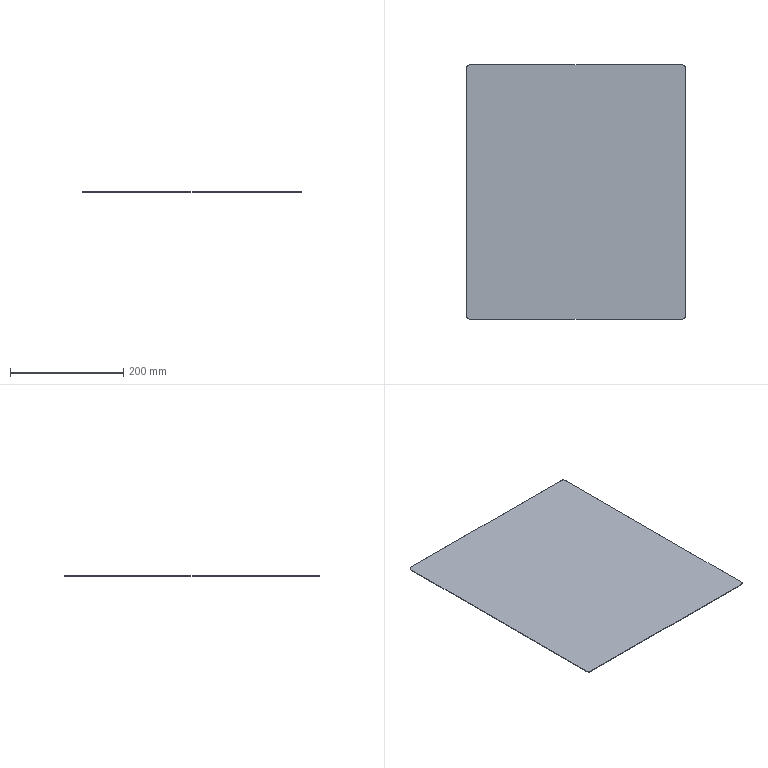Part | STEP file | PC board | 1 solid | 10 faces | box 386 x 450 x 1 mm | volume 173679 mm3 | plane 6 | cylinder 4 | commonest cylinder face diameters 10 x4
STEP:
#1=CARTESIAN_POINT('',(0.,0.,0.));
#2=DIRECTION('',(0.,0.,1.));
#3=DIRECTION('',(1.,0.,0.));
#4=AXIS2_PLACEMENT_3D('',#1,#2,#3);
#5=CARTESIAN_POINT('',(-193.,220.,0.5));
#6=VERTEX_POINT('',#5);
#7=CARTESIAN_POINT('',(-193.,-220.,0.5));
#8=VERTEX_POINT('',#7);
#9=CARTESIAN_POINT('',(-193.,225.,0.5));
#10=DIRECTION('',(0.,-1.,0.));
#11=VECTOR('',#10,1.);
#12=LINE('',#9,#11);
#13=CARTESIAN_POINT('',(-193.,225.,0.5));
#14=DIRECTION('',(1.,0.,0.));
#15=DIRECTION('',(0.,0.,-1.));
#16=AXIS2_PLACEMENT_3D('',#13,#14,#15);
#17=PLANE('',#16);
#18=CARTESIAN_POINT('',(0.,0.));
#19=DIRECTION('',(0.,-1.));
#20=VECTOR('',#19,1.);
#21=LINE('',#18,#20);
#22=(GEOMETRIC_REPRESENTATION_CONTEXT(2)PARAMETRIC_REPRESENTATION_CONTEXT()REPRESENTATION_CONTEXT('',''));
#23=DEFINITIONAL_REPRESENTATION('',(#21),#22);
#24=PCURVE('',#17,#23);
#25=CARTESIAN_POINT('',(193.,225.,0.5));
#26=DIRECTION('',(0.,0.,-1.));
#27=DIRECTION('',(-1.,0.,0.));
#28=AXIS2_PLACEMENT_3D('',#25,#26,#27);
#29=PLANE('',#28);
#30=CARTESIAN_POINT('',(386.,0.));
#31=DIRECTION('',(0.,-1.));
#32=VECTOR('',#31,1.);
#33=LINE('',#30,#32);
#34=(GEOMETRIC_REPRESENTATION_CONTEXT(2)PARAMETRIC_REPRESENTATION_CONTEXT()REPRESENTATION_CONTEXT('',''));
#35=DEFINITIONAL_REPRESENTATION('',(#33),#34);
#36=PCURVE('',#29,#35);
#37=SURFACE_CURVE('',#12,(#24,#36),.PCURVE_S1.);
#38=EDGE_CURVE('',#6,#8,#37,.T.);
#39=ORIENTED_EDGE('',*,*,#38,.F.);
#40=CARTESIAN_POINT('',(-193.,220.,-0.5));
#41=VERTEX_POINT('',#40);
#42=CARTESIAN_POINT('',(-193.,220.,-0.5));
#43=DIRECTION('',(0.,0.,-1.));
#44=VECTOR('',#43,1.);
#45=LINE('',#42,#44);
#46=CARTESIAN_POINT('',(1.,-5.));
#47=DIRECTION('',(1.,0.));
#48=VECTOR('',#47,1.);
#49=LINE('',#46,#48);
#50=(GEOMETRIC_REPRESENTATION_CONTEXT(2)PARAMETRIC_REPRESENTATION_CONTEXT()REPRESENTATION_CONTEXT('',''));
#51=DEFINITIONAL_REPRESENTATION('',(#49),#50);
#52=PCURVE('',#17,#51);
#53=CARTESIAN_POINT('',(-188.,220.,0.));
#54=DIRECTION('',(0.,0.,-1.));
#55=DIRECTION('',(-1.,0.,0.));
#56=AXIS2_PLACEMENT_3D('',#53,#54,#55);
#57=CYLINDRICAL_SURFACE('',#56,5.);
#58=CARTESIAN_POINT('',(0.,0.5));
#59=DIRECTION('',(0.,1.));
#60=VECTOR('',#59,1.);
#61=LINE('',#58,#60);
#62=(GEOMETRIC_REPRESENTATION_CONTEXT(2)PARAMETRIC_REPRESENTATION_CONTEXT()REPRESENTATION_CONTEXT('',''));
#63=DEFINITIONAL_REPRESENTATION('',(#61),#62);
#64=PCURVE('',#57,#63);
#65=SURFACE_CURVE('',#45,(#52,#64),.PCURVE_S1.);
#66=EDGE_CURVE('',#6,#41,#65,.T.);
#67=ORIENTED_EDGE('',*,*,#66,.T.);
#68=CARTESIAN_POINT('',(-193.,-220.,-0.5));
#69=VERTEX_POINT('',#68);
#70=CARTESIAN_POINT('',(-193.,225.,-0.5));
#71=DIRECTION('',(0.,-1.,0.));
#72=VECTOR('',#71,1.);
#73=LINE('',#70,#72);
#74=CARTESIAN_POINT('',(1.,0.));
#75=DIRECTION('',(0.,-1.));
#76=VECTOR('',#75,1.);
#77=LINE('',#74,#76);
#78=(GEOMETRIC_REPRESENTATION_CONTEXT(2)PARAMETRIC_REPRESENTATION_CONTEXT()REPRESENTATION_CONTEXT('',''));
#79=DEFINITIONAL_REPRESENTATION('',(#77),#78);
#80=PCURVE('',#17,#79);
#81=CARTESIAN_POINT('',(193.,225.,-0.5));
#82=DIRECTION('',(0.,0.,1.));
#83=DIRECTION('',(1.,0.,0.));
#84=AXIS2_PLACEMENT_3D('',#81,#82,#83);
#85=PLANE('',#84);
#86=CARTESIAN_POINT('',(-386.,0.));
#87=DIRECTION('',(0.,-1.));
#88=VECTOR('',#87,1.);
#89=LINE('',#86,#88);
#90=(GEOMETRIC_REPRESENTATION_CONTEXT(2)PARAMETRIC_REPRESENTATION_CONTEXT()REPRESENTATION_CONTEXT('',''));
#91=DEFINITIONAL_REPRESENTATION('',(#89),#90);
#92=PCURVE('',#85,#91);
#93=SURFACE_CURVE('',#73,(#80,#92),.PCURVE_S1.);
#94=EDGE_CURVE('',#41,#69,#93,.T.);
#95=ORIENTED_EDGE('',*,*,#94,.T.);
#96=CARTESIAN_POINT('',(-193.,-220.,0.5));
#97=DIRECTION('',(0.,0.,1.));
#98=VECTOR('',#97,1.);
#99=LINE('',#96,#98);
#100=CARTESIAN_POINT('',(0.,-445.));
#101=DIRECTION('',(-1.,0.));
#102=VECTOR('',#101,1.);
#103=LINE('',#100,#102);
#104=(GEOMETRIC_REPRESENTATION_CONTEXT(2)PARAMETRIC_REPRESENTATION_CONTEXT()REPRESENTATION_CONTEXT('',''));
#105=DEFINITIONAL_REPRESENTATION('',(#103),#104);
#106=PCURVE('',#17,#105);
#107=CARTESIAN_POINT('',(-188.,-220.,0.5));
#108=DIRECTION('',(0.,0.,1.));
#109=DIRECTION('',(1.,0.,0.));
#110=AXIS2_PLACEMENT_3D('',#107,#108,#109);
#111=CYLINDRICAL_SURFACE('',#110,5.);
#112=CARTESIAN_POINT('',(3.142,0.));
#113=DIRECTION('',(0.,1.));
#114=VECTOR('',#113,1.);
#115=LINE('',#112,#114);
#116=(GEOMETRIC_REPRESENTATION_CONTEXT(2)PARAMETRIC_REPRESENTATION_CONTEXT()REPRESENTATION_CONTEXT('',''));
#117=DEFINITIONAL_REPRESENTATION('',(#115),#116);
#118=PCURVE('',#111,#117);
#119=SURFACE_CURVE('',#99,(#106,#118),.PCURVE_S1.);
#120=EDGE_CURVE('',#69,#8,#119,.T.);
#121=ORIENTED_EDGE('',*,*,#120,.T.);
#122=EDGE_LOOP('',(#39,#67,#95,#121));
#123=FACE_BOUND('',#122,.T.);
#124=ADVANCED_FACE('',(#123),#17,.F.);
#125=CARTESIAN_POINT('',(193.,220.,0.5));
#126=VERTEX_POINT('',#125);
#127=CARTESIAN_POINT('',(193.,-220.,0.5));
#128=VERTEX_POINT('',#127);
#129=CARTESIAN_POINT('',(193.,225.,0.5));
#130=DIRECTION('',(0.,-1.,0.));
#131=VECTOR('',#130,1.);
#132=LINE('',#129,#131);
#133=CARTESIAN_POINT('',(0.,0.));
#134=DIRECTION('',(0.,-1.));
#135=VECTOR('',#134,1.);
#136=LINE('',#133,#135);
#137=(GEOMETRIC_REPRESENTATION_CONTEXT(2)PARAMETRIC_REPRESENTATION_CONTEXT()REPRESENTATION_CONTEXT('',''));
#138=DEFINITIONAL_REPRESENTATION('',(#136),#137);
#139=PCURVE('',#29,#138);
#140=CARTESIAN_POINT('',(193.,225.,0.5));
#141=DIRECTION('',(-1.,0.,0.));
#142=DIRECTION('',(0.,0.,1.));
#143=AXIS2_PLACEMENT_3D('',#140,#141,#142);
#144=PLANE('',#143);
#145=CARTESIAN_POINT('',(0.,0.));
#146=DIRECTION('',(0.,-1.));
#147=VECTOR('',#146,1.);
#148=LINE('',#145,#147);
#149=(GEOMETRIC_REPRESENTATION_CONTEXT(2)PARAMETRIC_REPRESENTATION_CONTEXT()REPRESENTATION_CONTEXT('',''));
#150=DEFINITIONAL_REPRESENTATION('',(#148),#149);
#151=PCURVE('',#144,#150);
#152=SURFACE_CURVE('',#132,(#139,#151),.PCURVE_S1.);
#153=EDGE_CURVE('',#126,#128,#152,.T.);
#154=ORIENTED_EDGE('',*,*,#153,.F.);
#155=CARTESIAN_POINT('',(188.,225.,0.5));
#156=VERTEX_POINT('',#155);
#157=CARTESIAN_POINT('',(188.,220.,0.5));
#158=DIRECTION('',(0.,0.,1.));
#159=DIRECTION('',(-1.,0.,0.));
#160=AXIS2_PLACEMENT_3D('',#157,#158,#159);
#161=CIRCLE('',#160,5.);
#162=CARTESIAN_POINT('',(10.,-5.));
#163=CARTESIAN_POINT('',(10.,-13.66));
#164=CARTESIAN_POINT('',(2.5,-9.33));
#165=CARTESIAN_POINT('',(-5.,-5.));
#166=CARTESIAN_POINT('',(2.5,-0.6699));
#167=CARTESIAN_POINT('',(10.,3.66));
#168=CARTESIAN_POINT('',(10.,-5.));
#169=(BOUNDED_CURVE()B_SPLINE_CURVE(2,(#162,#163,#164,#165,#166,#167,#168),.UNSPECIFIED.,.T.,.F.)B_SPLINE_CURVE_WITH_KNOTS((1,2,2,2,2,1),(-2.094,0.,2.094,4.189,6.283,8.378),.UNSPECIFIED.)CURVE()GEOMETRIC_REPRESENTATION_ITEM()RATIONAL_B_SPLINE_CURVE((1.,0.5,1.,0.5,1.,0.5,1.))REPRESENTATION_ITEM(''));
#170=(GEOMETRIC_REPRESENTATION_CONTEXT(2)PARAMETRIC_REPRESENTATION_CONTEXT()REPRESENTATION_CONTEXT('',''));
#171=DEFINITIONAL_REPRESENTATION('',(#169),#170);
#172=PCURVE('',#29,#171);
#173=CARTESIAN_POINT('',(188.,220.,0.));
#174=DIRECTION('',(0.,0.,1.));
#175=DIRECTION('',(1.,0.,0.));
#176=AXIS2_PLACEMENT_3D('',#173,#174,#175);
#177=CYLINDRICAL_SURFACE('',#176,5.);
#178=CARTESIAN_POINT('',(-3.142,0.5));
#179=DIRECTION('',(1.,0.));
#180=VECTOR('',#179,1.);
#181=LINE('',#178,#180);
#182=(GEOMETRIC_REPRESENTATION_CONTEXT(2)PARAMETRIC_REPRESENTATION_CONTEXT()REPRESENTATION_CONTEXT('',''));
#183=DEFINITIONAL_REPRESENTATION('',(#181),#182);
#184=PCURVE('',#177,#183);
#185=SURFACE_CURVE('',#161,(#172,#184),.PCURVE_S1.);
#186=EDGE_CURVE('',#126,#156,#185,.T.);
#187=ORIENTED_EDGE('',*,*,#186,.T.);
#188=CARTESIAN_POINT('',(-188.,225.,0.5));
#189=VERTEX_POINT('',#188);
#190=CARTESIAN_POINT('',(193.,225.,0.5));
#191=DIRECTION('',(1.,0.,0.));
#192=VECTOR('',#191,1.);
#193=LINE('',#190,#192);
#194=CARTESIAN_POINT('',(0.,0.));
#195=DIRECTION('',(-1.,0.));
#196=VECTOR('',#195,1.);
#197=LINE('',#194,#196);
#198=(GEOMETRIC_REPRESENTATION_CONTEXT(2)PARAMETRIC_REPRESENTATION_CONTEXT()REPRESENTATION_CONTEXT('',''));
#199=DEFINITIONAL_REPRESENTATION('',(#197),#198);
#200=PCURVE('',#29,#199);
#201=CARTESIAN_POINT('',(0.,225.,0.));
#202=DIRECTION('',(0.,1.,0.));
#203=DIRECTION('',(0.,0.,1.));
#204=AXIS2_PLACEMENT_3D('',#201,#202,#203);
#205=PLANE('',#204);
#206=CARTESIAN_POINT('',(0.5,193.));
#207=DIRECTION('',(0.,1.));
#208=VECTOR('',#207,1.);
#209=LINE('',#206,#208);
#210=(GEOMETRIC_REPRESENTATION_CONTEXT(2)PARAMETRIC_REPRESENTATION_CONTEXT()REPRESENTATION_CONTEXT('',''));
#211=DEFINITIONAL_REPRESENTATION('',(#209),#210);
#212=PCURVE('',#205,#211);
#213=SURFACE_CURVE('',#193,(#200,#212),.PCURVE_S1.);
#214=EDGE_CURVE('',#189,#156,#213,.T.);
#215=ORIENTED_EDGE('',*,*,#214,.F.);
#216=CARTESIAN_POINT('',(-188.,220.,0.5));
#217=DIRECTION('',(0.,0.,1.));
#218=DIRECTION('',(-1.,0.,0.));
#219=AXIS2_PLACEMENT_3D('',#216,#217,#218);
#220=CIRCLE('',#219,5.);
#221=CARTESIAN_POINT('',(386.,-5.));
#222=CARTESIAN_POINT('',(386.,-13.66));
#223=CARTESIAN_POINT('',(378.5,-9.33));
#224=CARTESIAN_POINT('',(371.,-5.));
#225=CARTESIAN_POINT('',(378.5,-0.6699));
#226=CARTESIAN_POINT('',(386.,3.66));
#227=CARTESIAN_POINT('',(386.,-5.));
#228=(BOUNDED_CURVE()B_SPLINE_CURVE(2,(#221,#222,#223,#224,#225,#226,#227),.UNSPECIFIED.,.T.,.F.)B_SPLINE_CURVE_WITH_KNOTS((1,2,2,2,2,1),(-2.094,0.,2.094,4.189,6.283,8.378),.UNSPECIFIED.)CURVE()GEOMETRIC_REPRESENTATION_ITEM()RATIONAL_B_SPLINE_CURVE((1.,0.5,1.,0.5,1.,0.5,1.))REPRESENTATION_ITEM(''));
#229=(GEOMETRIC_REPRESENTATION_CONTEXT(2)PARAMETRIC_REPRESENTATION_CONTEXT()REPRESENTATION_CONTEXT('',''));
#230=DEFINITIONAL_REPRESENTATION('',(#228),#229);
#231=PCURVE('',#29,#230);
#232=CARTESIAN_POINT('',(6.283,-0.5));
#233=DIRECTION('',(-1.,0.));
#234=VECTOR('',#233,1.);
#235=LINE('',#232,#234);
#236=(GEOMETRIC_REPRESENTATION_CONTEXT(2)PARAMETRIC_REPRESENTATION_CONTEXT()REPRESENTATION_CONTEXT('',''));
#237=DEFINITIONAL_REPRESENTATION('',(#235),#236);
#238=PCURVE('',#57,#237);
#239=SURFACE_CURVE('',#220,(#231,#238),.PCURVE_S1.);
#240=EDGE_CURVE('',#189,#6,#239,.T.);
#241=ORIENTED_EDGE('',*,*,#240,.T.);
#242=ORIENTED_EDGE('',*,*,#38,.T.);
#243=CARTESIAN_POINT('',(-188.,-225.,0.5));
#244=VERTEX_POINT('',#243);
#245=CARTESIAN_POINT('',(-188.,-220.,0.5));
#246=DIRECTION('',(0.,0.,1.));
#247=DIRECTION('',(-1.,0.,0.));
#248=AXIS2_PLACEMENT_3D('',#245,#246,#247);
#249=CIRCLE('',#248,5.);
#250=CARTESIAN_POINT('',(386.,-445.));
#251=CARTESIAN_POINT('',(386.,-453.66));
#252=CARTESIAN_POINT('',(378.5,-449.33));
#253=CARTESIAN_POINT('',(371.,-445.));
#254=CARTESIAN_POINT('',(378.5,-440.67));
#255=CARTESIAN_POINT('',(386.,-436.34));
#256=CARTESIAN_POINT('',(386.,-445.));
#257=(BOUNDED_CURVE()B_SPLINE_CURVE(2,(#250,#251,#252,#253,#254,#255,#256),.UNSPECIFIED.,.T.,.F.)B_SPLINE_CURVE_WITH_KNOTS((1,2,2,2,2,1),(-2.094,0.,2.094,4.189,6.283,8.378),.UNSPECIFIED.)CURVE()GEOMETRIC_REPRESENTATION_ITEM()RATIONAL_B_SPLINE_CURVE((1.,0.5,1.,0.5,1.,0.5,1.))REPRESENTATION_ITEM(''));
#258=(GEOMETRIC_REPRESENTATION_CONTEXT(2)PARAMETRIC_REPRESENTATION_CONTEXT()REPRESENTATION_CONTEXT('',''));
#259=DEFINITIONAL_REPRESENTATION('',(#257),#258);
#260=PCURVE('',#29,#259);
#261=CARTESIAN_POINT('',(3.142,0.));
#262=DIRECTION('',(1.,0.));
#263=VECTOR('',#262,1.);
#264=LINE('',#261,#263);
#265=(GEOMETRIC_REPRESENTATION_CONTEXT(2)PARAMETRIC_REPRESENTATION_CONTEXT()REPRESENTATION_CONTEXT('',''));
#266=DEFINITIONAL_REPRESENTATION('',(#264),#265);
#267=PCURVE('',#111,#266);
#268=SURFACE_CURVE('',#249,(#260,#267),.PCURVE_S1.);
#269=EDGE_CURVE('',#8,#244,#268,.T.);
#270=ORIENTED_EDGE('',*,*,#269,.T.);
#271=CARTESIAN_POINT('',(188.,-225.,0.5));
#272=VERTEX_POINT('',#271);
#273=CARTESIAN_POINT('',(193.,-225.,0.5));
#274=DIRECTION('',(1.,0.,0.));
#275=VECTOR('',#274,1.);
#276=LINE('',#273,#275);
#277=CARTESIAN_POINT('',(0.,-450.));
#278=DIRECTION('',(-1.,0.));
#279=VECTOR('',#278,1.);
#280=LINE('',#277,#279);
#281=(GEOMETRIC_REPRESENTATION_CONTEXT(2)PARAMETRIC_REPRESENTATION_CONTEXT()REPRESENTATION_CONTEXT('',''));
#282=DEFINITIONAL_REPRESENTATION('',(#280),#281);
#283=PCURVE('',#29,#282);
#284=CARTESIAN_POINT('',(0.,-225.,0.));
#285=DIRECTION('',(0.,1.,0.));
#286=DIRECTION('',(0.,0.,1.));
#287=AXIS2_PLACEMENT_3D('',#284,#285,#286);
#288=PLANE('',#287);
#289=CARTESIAN_POINT('',(0.5,193.));
#290=DIRECTION('',(0.,1.));
#291=VECTOR('',#290,1.);
#292=LINE('',#289,#291);
#293=(GEOMETRIC_REPRESENTATION_CONTEXT(2)PARAMETRIC_REPRESENTATION_CONTEXT()REPRESENTATION_CONTEXT('',''));
#294=DEFINITIONAL_REPRESENTATION('',(#292),#293);
#295=PCURVE('',#288,#294);
#296=SURFACE_CURVE('',#276,(#283,#295),.PCURVE_S1.);
#297=EDGE_CURVE('',#244,#272,#296,.T.);
#298=ORIENTED_EDGE('',*,*,#297,.T.);
#299=CARTESIAN_POINT('',(188.,-220.,0.5));
#300=DIRECTION('',(0.,0.,1.));
#301=DIRECTION('',(-1.,0.,0.));
#302=AXIS2_PLACEMENT_3D('',#299,#300,#301);
#303=CIRCLE('',#302,5.);
#304=CARTESIAN_POINT('',(10.,-445.));
#305=CARTESIAN_POINT('',(10.,-453.66));
#306=CARTESIAN_POINT('',(2.5,-449.33));
#307=CARTESIAN_POINT('',(-5.,-445.));
#308=CARTESIAN_POINT('',(2.5,-440.67));
#309=CARTESIAN_POINT('',(10.,-436.34));
#310=CARTESIAN_POINT('',(10.,-445.));
#311=(BOUNDED_CURVE()B_SPLINE_CURVE(2,(#304,#305,#306,#307,#308,#309,#310),.UNSPECIFIED.,.T.,.F.)B_SPLINE_CURVE_WITH_KNOTS((1,2,2,2,2,1),(-2.094,0.,2.094,4.189,6.283,8.378),.UNSPECIFIED.)CURVE()GEOMETRIC_REPRESENTATION_ITEM()RATIONAL_B_SPLINE_CURVE((1.,0.5,1.,0.5,1.,0.5,1.))REPRESENTATION_ITEM(''));
#312=(GEOMETRIC_REPRESENTATION_CONTEXT(2)PARAMETRIC_REPRESENTATION_CONTEXT()REPRESENTATION_CONTEXT('',''));
#313=DEFINITIONAL_REPRESENTATION('',(#311),#312);
#314=PCURVE('',#29,#313);
#315=CARTESIAN_POINT('',(188.,-220.,0.5));
#316=DIRECTION('',(0.,0.,-1.));
#317=DIRECTION('',(-1.,0.,0.));
#318=AXIS2_PLACEMENT_3D('',#315,#316,#317);
#319=CYLINDRICAL_SURFACE('',#318,5.);
#320=CARTESIAN_POINT('',(6.283,0.));
#321=DIRECTION('',(-1.,0.));
#322=VECTOR('',#321,1.);
#323=LINE('',#320,#322);
#324=(GEOMETRIC_REPRESENTATION_CONTEXT(2)PARAMETRIC_REPRESENTATION_CONTEXT()REPRESENTATION_CONTEXT('',''));
#325=DEFINITIONAL_REPRESENTATION('',(#323),#324);
#326=PCURVE('',#319,#325);
#327=SURFACE_CURVE('',#303,(#314,#326),.PCURVE_S1.);
#328=EDGE_CURVE('',#272,#128,#327,.T.);
#329=ORIENTED_EDGE('',*,*,#328,.T.);
#330=EDGE_LOOP('',(#154,#187,#215,#241,#242,#270,#298,#329));
#331=FACE_BOUND('',#330,.T.);
#332=ADVANCED_FACE('',(#331),#29,.F.);
#333=CARTESIAN_POINT('',(193.,220.,-0.5));
#334=VERTEX_POINT('',#333);
#335=CARTESIAN_POINT('',(193.,-220.,-0.5));
#336=VERTEX_POINT('',#335);
#337=CARTESIAN_POINT('',(193.,225.,-0.5));
#338=DIRECTION('',(0.,-1.,0.));
#339=VECTOR('',#338,1.);
#340=LINE('',#337,#339);
#341=CARTESIAN_POINT('',(-1.,0.));
#342=DIRECTION('',(0.,-1.));
#343=VECTOR('',#342,1.);
#344=LINE('',#341,#343);
#345=(GEOMETRIC_REPRESENTATION_CONTEXT(2)PARAMETRIC_REPRESENTATION_CONTEXT()REPRESENTATION_CONTEXT('',''));
#346=DEFINITIONAL_REPRESENTATION('',(#344),#345);
#347=PCURVE('',#144,#346);
#348=CARTESIAN_POINT('',(0.,0.));
#349=DIRECTION('',(0.,-1.));
#350=VECTOR('',#349,1.);
#351=LINE('',#348,#350);
#352=(GEOMETRIC_REPRESENTATION_CONTEXT(2)PARAMETRIC_REPRESENTATION_CONTEXT()REPRESENTATION_CONTEXT('',''));
#353=DEFINITIONAL_REPRESENTATION('',(#351),#352);
#354=PCURVE('',#85,#353);
#355=SURFACE_CURVE('',#340,(#347,#354),.PCURVE_S1.);
#356=EDGE_CURVE('',#334,#336,#355,.T.);
#357=ORIENTED_EDGE('',*,*,#356,.F.);
#358=CARTESIAN_POINT('',(193.,220.,0.5));
#359=DIRECTION('',(0.,0.,1.));
#360=VECTOR('',#359,1.);
#361=LINE('',#358,#360);
#362=CARTESIAN_POINT('',(0.,-5.));
#363=DIRECTION('',(1.,0.));
#364=VECTOR('',#363,1.);
#365=LINE('',#362,#364);
#366=(GEOMETRIC_REPRESENTATION_CONTEXT(2)PARAMETRIC_REPRESENTATION_CONTEXT()REPRESENTATION_CONTEXT('',''));
#367=DEFINITIONAL_REPRESENTATION('',(#365),#366);
#368=PCURVE('',#144,#367);
#369=CARTESIAN_POINT('',(0.,0.5));
#370=DIRECTION('',(0.,1.));
#371=VECTOR('',#370,1.);
#372=LINE('',#369,#371);
#373=(GEOMETRIC_REPRESENTATION_CONTEXT(2)PARAMETRIC_REPRESENTATION_CONTEXT()REPRESENTATION_CONTEXT('',''));
#374=DEFINITIONAL_REPRESENTATION('',(#372),#373);
#375=PCURVE('',#177,#374);
#376=SURFACE_CURVE('',#361,(#368,#375),.PCURVE_S1.);
#377=EDGE_CURVE('',#334,#126,#376,.T.);
#378=ORIENTED_EDGE('',*,*,#377,.T.);
#379=ORIENTED_EDGE('',*,*,#153,.T.);
#380=CARTESIAN_POINT('',(193.,-220.,0.5));
#381=DIRECTION('',(0.,0.,-1.));
#382=VECTOR('',#381,1.);
#383=LINE('',#380,#382);
#384=CARTESIAN_POINT('',(0.,-445.));
#385=DIRECTION('',(-1.,0.));
#386=VECTOR('',#385,1.);
#387=LINE('',#384,#386);
#388=(GEOMETRIC_REPRESENTATION_CONTEXT(2)PARAMETRIC_REPRESENTATION_CONTEXT()REPRESENTATION_CONTEXT('',''));
#389=DEFINITIONAL_REPRESENTATION('',(#387),#388);
#390=PCURVE('',#144,#389);
#391=CARTESIAN_POINT('',(3.142,0.));
#392=DIRECTION('',(0.,1.));
#393=VECTOR('',#392,1.);
#394=LINE('',#391,#393);
#395=(GEOMETRIC_REPRESENTATION_CONTEXT(2)PARAMETRIC_REPRESENTATION_CONTEXT()REPRESENTATION_CONTEXT('',''));
#396=DEFINITIONAL_REPRESENTATION('',(#394),#395);
#397=PCURVE('',#319,#396);
#398=SURFACE_CURVE('',#383,(#390,#397),.PCURVE_S1.);
#399=EDGE_CURVE('',#128,#336,#398,.T.);
#400=ORIENTED_EDGE('',*,*,#399,.T.);
#401=EDGE_LOOP('',(#357,#378,#379,#400));
#402=FACE_BOUND('',#401,.T.);
#403=ADVANCED_FACE('',(#402),#144,.F.);
#404=CARTESIAN_POINT('',(188.,225.,-0.5));
#405=VERTEX_POINT('',#404);
#406=CARTESIAN_POINT('',(-188.,225.,-0.5));
#407=VERTEX_POINT('',#406);
#408=CARTESIAN_POINT('',(193.,225.,-0.5));
#409=DIRECTION('',(-1.,0.,0.));
#410=VECTOR('',#409,1.);
#411=LINE('',#408,#410);
#412=CARTESIAN_POINT('',(0.,0.));
#413=DIRECTION('',(-1.,0.));
#414=VECTOR('',#413,1.);
#415=LINE('',#412,#414);
#416=(GEOMETRIC_REPRESENTATION_CONTEXT(2)PARAMETRIC_REPRESENTATION_CONTEXT()REPRESENTATION_CONTEXT('',''));
#417=DEFINITIONAL_REPRESENTATION('',(#415),#416);
#418=PCURVE('',#85,#417);
#419=CARTESIAN_POINT('',(-0.5,193.));
#420=DIRECTION('',(0.,-1.));
#421=VECTOR('',#420,1.);
#422=LINE('',#419,#421);
#423=(GEOMETRIC_REPRESENTATION_CONTEXT(2)PARAMETRIC_REPRESENTATION_CONTEXT()REPRESENTATION_CONTEXT('',''));
#424=DEFINITIONAL_REPRESENTATION('',(#422),#423);
#425=PCURVE('',#205,#424);
#426=SURFACE_CURVE('',#411,(#418,#425),.PCURVE_S1.);
#427=EDGE_CURVE('',#405,#407,#426,.T.);
#428=ORIENTED_EDGE('',*,*,#427,.F.);
#429=CARTESIAN_POINT('',(188.,220.,-0.5));
#430=DIRECTION('',(0.,0.,-1.));
#431=DIRECTION('',(1.,0.,0.));
#432=AXIS2_PLACEMENT_3D('',#429,#430,#431);
#433=CIRCLE('',#432,5.);
#434=CARTESIAN_POINT('',(0.,-5.));
#435=CARTESIAN_POINT('',(0.,-13.66));
#436=CARTESIAN_POINT('',(-7.5,-9.33));
#437=CARTESIAN_POINT('',(-15.,-5.));
#438=CARTESIAN_POINT('',(-7.5,-0.6699));
#439=CARTESIAN_POINT('',(0.,3.66));
#440=CARTESIAN_POINT('',(0.,-5.));
#441=(BOUNDED_CURVE()B_SPLINE_CURVE(2,(#434,#435,#436,#437,#438,#439,#440),.UNSPECIFIED.,.T.,.F.)B_SPLINE_CURVE_WITH_KNOTS((1,2,2,2,2,1),(-2.094,0.,2.094,4.189,6.283,8.378),.UNSPECIFIED.)CURVE()GEOMETRIC_REPRESENTATION_ITEM()RATIONAL_B_SPLINE_CURVE((1.,0.5,1.,0.5,1.,0.5,1.))REPRESENTATION_ITEM(''));
#442=(GEOMETRIC_REPRESENTATION_CONTEXT(2)PARAMETRIC_REPRESENTATION_CONTEXT()REPRESENTATION_CONTEXT('',''));
#443=DEFINITIONAL_REPRESENTATION('',(#441),#442);
#444=PCURVE('',#85,#443);
#445=CARTESIAN_POINT('',(6.283,-0.5));
#446=DIRECTION('',(-1.,0.));
#447=VECTOR('',#446,1.);
#448=LINE('',#445,#447);
#449=(GEOMETRIC_REPRESENTATION_CONTEXT(2)PARAMETRIC_REPRESENTATION_CONTEXT()REPRESENTATION_CONTEXT('',''));
#450=DEFINITIONAL_REPRESENTATION('',(#448),#449);
#451=PCURVE('',#177,#450);
#452=SURFACE_CURVE('',#433,(#444,#451),.PCURVE_S1.);
#453=EDGE_CURVE('',#405,#334,#452,.T.);
#454=ORIENTED_EDGE('',*,*,#453,.T.);
#455=ORIENTED_EDGE('',*,*,#356,.T.);
#456=CARTESIAN_POINT('',(188.,-225.,-0.5));
#457=VERTEX_POINT('',#456);
#458=CARTESIAN_POINT('',(188.,-220.,-0.5));
#459=DIRECTION('',(0.,0.,-1.));
#460=DIRECTION('',(1.,0.,0.));
#461=AXIS2_PLACEMENT_3D('',#458,#459,#460);
#462=CIRCLE('',#461,5.);
#463=CARTESIAN_POINT('',(0.,-445.));
#464=CARTESIAN_POINT('',(0.,-453.66));
#465=CARTESIAN_POINT('',(-7.5,-449.33));
#466=CARTESIAN_POINT('',(-15.,-445.));
#467=CARTESIAN_POINT('',(-7.5,-440.67));
#468=CARTESIAN_POINT('',(0.,-436.34));
#469=CARTESIAN_POINT('',(0.,-445.));
#470=(BOUNDED_CURVE()B_SPLINE_CURVE(2,(#463,#464,#465,#466,#467,#468,#469),.UNSPECIFIED.,.T.,.F.)B_SPLINE_CURVE_WITH_KNOTS((1,2,2,2,2,1),(-2.094,0.,2.094,4.189,6.283,8.378),.UNSPECIFIED.)CURVE()GEOMETRIC_REPRESENTATION_ITEM()RATIONAL_B_SPLINE_CURVE((1.,0.5,1.,0.5,1.,0.5,1.))REPRESENTATION_ITEM(''));
#471=(GEOMETRIC_REPRESENTATION_CONTEXT(2)PARAMETRIC_REPRESENTATION_CONTEXT()REPRESENTATION_CONTEXT('',''));
#472=DEFINITIONAL_REPRESENTATION('',(#470),#471);
#473=PCURVE('',#85,#472);
#474=CARTESIAN_POINT('',(3.142,1.));
#475=DIRECTION('',(1.,0.));
#476=VECTOR('',#475,1.);
#477=LINE('',#474,#476);
#478=(GEOMETRIC_REPRESENTATION_CONTEXT(2)PARAMETRIC_REPRESENTATION_CONTEXT()REPRESENTATION_CONTEXT('',''));
#479=DEFINITIONAL_REPRESENTATION('',(#477),#478);
#480=PCURVE('',#319,#479);
#481=SURFACE_CURVE('',#462,(#473,#480),.PCURVE_S1.);
#482=EDGE_CURVE('',#336,#457,#481,.T.);
#483=ORIENTED_EDGE('',*,*,#482,.T.);
#484=CARTESIAN_POINT('',(-188.,-225.,-0.5));
#485=VERTEX_POINT('',#484);
#486=CARTESIAN_POINT('',(193.,-225.,-0.5));
#487=DIRECTION('',(-1.,0.,0.));
#488=VECTOR('',#487,1.);
#489=LINE('',#486,#488);
#490=CARTESIAN_POINT('',(0.,-450.));
#491=DIRECTION('',(-1.,0.));
#492=VECTOR('',#491,1.);
#493=LINE('',#490,#492);
#494=(GEOMETRIC_REPRESENTATION_CONTEXT(2)PARAMETRIC_REPRESENTATION_CONTEXT()REPRESENTATION_CONTEXT('',''));
#495=DEFINITIONAL_REPRESENTATION('',(#493),#494);
#496=PCURVE('',#85,#495);
#497=CARTESIAN_POINT('',(-0.5,193.));
#498=DIRECTION('',(0.,-1.));
#499=VECTOR('',#498,1.);
#500=LINE('',#497,#499);
#501=(GEOMETRIC_REPRESENTATION_CONTEXT(2)PARAMETRIC_REPRESENTATION_CONTEXT()REPRESENTATION_CONTEXT('',''));
#502=DEFINITIONAL_REPRESENTATION('',(#500),#501);
#503=PCURVE('',#288,#502);
#504=SURFACE_CURVE('',#489,(#496,#503),.PCURVE_S1.);
#505=EDGE_CURVE('',#457,#485,#504,.T.);
#506=ORIENTED_EDGE('',*,*,#505,.T.);
#507=CARTESIAN_POINT('',(-188.,-220.,-0.5));
#508=DIRECTION('',(0.,0.,-1.));
#509=DIRECTION('',(1.,0.,0.));
#510=AXIS2_PLACEMENT_3D('',#507,#508,#509);
#511=CIRCLE('',#510,5.);
#512=CARTESIAN_POINT('',(-376.,-445.));
#513=CARTESIAN_POINT('',(-376.,-453.66));
#514=CARTESIAN_POINT('',(-383.5,-449.33));
#515=CARTESIAN_POINT('',(-391.,-445.));
#516=CARTESIAN_POINT('',(-383.5,-440.67));
#517=CARTESIAN_POINT('',(-376.,-436.34));
#518=CARTESIAN_POINT('',(-376.,-445.));
#519=(BOUNDED_CURVE()B_SPLINE_CURVE(2,(#512,#513,#514,#515,#516,#517,#518),.UNSPECIFIED.,.T.,.F.)B_SPLINE_CURVE_WITH_KNOTS((1,2,2,2,2,1),(-2.094,0.,2.094,4.189,6.283,8.378),.UNSPECIFIED.)CURVE()GEOMETRIC_REPRESENTATION_ITEM()RATIONAL_B_SPLINE_CURVE((1.,0.5,1.,0.5,1.,0.5,1.))REPRESENTATION_ITEM(''));
#520=(GEOMETRIC_REPRESENTATION_CONTEXT(2)PARAMETRIC_REPRESENTATION_CONTEXT()REPRESENTATION_CONTEXT('',''));
#521=DEFINITIONAL_REPRESENTATION('',(#519),#520);
#522=PCURVE('',#85,#521);
#523=CARTESIAN_POINT('',(6.283,-1.));
#524=DIRECTION('',(-1.,0.));
#525=VECTOR('',#524,1.);
#526=LINE('',#523,#525);
#527=(GEOMETRIC_REPRESENTATION_CONTEXT(2)PARAMETRIC_REPRESENTATION_CONTEXT()REPRESENTATION_CONTEXT('',''));
#528=DEFINITIONAL_REPRESENTATION('',(#526),#527);
#529=PCURVE('',#111,#528);
#530=SURFACE_CURVE('',#511,(#522,#529),.PCURVE_S1.);
#531=EDGE_CURVE('',#485,#69,#530,.T.);
#532=ORIENTED_EDGE('',*,*,#531,.T.);
#533=ORIENTED_EDGE('',*,*,#94,.F.);
#534=CARTESIAN_POINT('',(-188.,220.,-0.5));
#535=DIRECTION('',(0.,0.,-1.));
#536=DIRECTION('',(1.,0.,0.));
#537=AXIS2_PLACEMENT_3D('',#534,#535,#536);
#538=CIRCLE('',#537,5.);
#539=CARTESIAN_POINT('',(-376.,-5.));
#540=CARTESIAN_POINT('',(-376.,-13.66));
#541=CARTESIAN_POINT('',(-383.5,-9.33));
#542=CARTESIAN_POINT('',(-391.,-5.));
#543=CARTESIAN_POINT('',(-383.5,-0.6699));
#544=CARTESIAN_POINT('',(-376.,3.66));
#545=CARTESIAN_POINT('',(-376.,-5.));
#546=(BOUNDED_CURVE()B_SPLINE_CURVE(2,(#539,#540,#541,#542,#543,#544,#545),.UNSPECIFIED.,.T.,.F.)B_SPLINE_CURVE_WITH_KNOTS((1,2,2,2,2,1),(-2.094,0.,2.094,4.189,6.283,8.378),.UNSPECIFIED.)CURVE()GEOMETRIC_REPRESENTATION_ITEM()RATIONAL_B_SPLINE_CURVE((1.,0.5,1.,0.5,1.,0.5,1.))REPRESENTATION_ITEM(''));
#547=(GEOMETRIC_REPRESENTATION_CONTEXT(2)PARAMETRIC_REPRESENTATION_CONTEXT()REPRESENTATION_CONTEXT('',''));
#548=DEFINITIONAL_REPRESENTATION('',(#546),#547);
#549=PCURVE('',#85,#548);
#550=CARTESIAN_POINT('',(-3.142,0.5));
#551=DIRECTION('',(1.,0.));
#552=VECTOR('',#551,1.);
#553=LINE('',#550,#552);
#554=(GEOMETRIC_REPRESENTATION_CONTEXT(2)PARAMETRIC_REPRESENTATION_CONTEXT()REPRESENTATION_CONTEXT('',''));
#555=DEFINITIONAL_REPRESENTATION('',(#553),#554);
#556=PCURVE('',#57,#555);
#557=SURFACE_CURVE('',#538,(#549,#556),.PCURVE_S1.);
#558=EDGE_CURVE('',#41,#407,#557,.T.);
#559=ORIENTED_EDGE('',*,*,#558,.T.);
#560=EDGE_LOOP('',(#428,#454,#455,#483,#506,#532,#533,#559));
#561=FACE_BOUND('',#560,.T.);
#562=ADVANCED_FACE('',(#561),#85,.F.);
#563=ORIENTED_EDGE('',*,*,#214,.T.);
#564=CARTESIAN_POINT('',(188.,225.,-0.5));
#565=DIRECTION('',(0.,0.,-1.));
#566=VECTOR('',#565,1.);
#567=LINE('',#564,#566);
#568=CARTESIAN_POINT('',(-0.5,188.));
#569=DIRECTION('',(-1.,0.));
#570=VECTOR('',#569,1.);
#571=LINE('',#568,#570);
#572=(GEOMETRIC_REPRESENTATION_CONTEXT(2)PARAMETRIC_REPRESENTATION_CONTEXT()REPRESENTATION_CONTEXT('',''));
#573=DEFINITIONAL_REPRESENTATION('',(#571),#572);
#574=PCURVE('',#205,#573);
#575=CARTESIAN_POINT('',(1.571,-0.5));
#576=DIRECTION('',(0.,-1.));
#577=VECTOR('',#576,1.);
#578=LINE('',#575,#577);
#579=(GEOMETRIC_REPRESENTATION_CONTEXT(2)PARAMETRIC_REPRESENTATION_CONTEXT()REPRESENTATION_CONTEXT('',''));
#580=DEFINITIONAL_REPRESENTATION('',(#578),#579);
#581=PCURVE('',#177,#580);
#582=SURFACE_CURVE('',#567,(#574,#581),.PCURVE_S1.);
#583=EDGE_CURVE('',#156,#405,#582,.T.);
#584=ORIENTED_EDGE('',*,*,#583,.T.);
#585=ORIENTED_EDGE('',*,*,#427,.T.);
#586=CARTESIAN_POINT('',(-188.,225.,0.5));
#587=DIRECTION('',(0.,0.,1.));
#588=VECTOR('',#587,1.);
#589=LINE('',#586,#588);
#590=CARTESIAN_POINT('',(0.5,-188.));
#591=DIRECTION('',(1.,0.));
#592=VECTOR('',#591,1.);
#593=LINE('',#590,#592);
#594=(GEOMETRIC_REPRESENTATION_CONTEXT(2)PARAMETRIC_REPRESENTATION_CONTEXT()REPRESENTATION_CONTEXT('',''));
#595=DEFINITIONAL_REPRESENTATION('',(#593),#594);
#596=PCURVE('',#205,#595);
#597=CARTESIAN_POINT('',(1.571,-0.5));
#598=DIRECTION('',(0.,-1.));
#599=VECTOR('',#598,1.);
#600=LINE('',#597,#599);
#601=(GEOMETRIC_REPRESENTATION_CONTEXT(2)PARAMETRIC_REPRESENTATION_CONTEXT()REPRESENTATION_CONTEXT('',''));
#602=DEFINITIONAL_REPRESENTATION('',(#600),#601);
#603=PCURVE('',#57,#602);
#604=SURFACE_CURVE('',#589,(#596,#603),.PCURVE_S1.);
#605=EDGE_CURVE('',#407,#189,#604,.T.);
#606=ORIENTED_EDGE('',*,*,#605,.T.);
#607=EDGE_LOOP('',(#563,#584,#585,#606));
#608=FACE_BOUND('',#607,.T.);
#609=ADVANCED_FACE('',(#608),#205,.T.);
#610=ORIENTED_EDGE('',*,*,#297,.F.);
#611=CARTESIAN_POINT('',(-188.,-225.,0.));
#612=DIRECTION('',(0.,0.,-1.));
#613=VECTOR('',#612,1.);
#614=LINE('',#611,#613);
#615=CARTESIAN_POINT('',(0.,-188.));
#616=DIRECTION('',(-1.,0.));
#617=VECTOR('',#616,1.);
#618=LINE('',#615,#617);
#619=(GEOMETRIC_REPRESENTATION_CONTEXT(2)PARAMETRIC_REPRESENTATION_CONTEXT()REPRESENTATION_CONTEXT('',''));
#620=DEFINITIONAL_REPRESENTATION('',(#618),#619);
#621=PCURVE('',#288,#620);
#622=CARTESIAN_POINT('',(4.712,-0.5));
#623=DIRECTION('',(0.,-1.));
#624=VECTOR('',#623,1.);
#625=LINE('',#622,#624);
#626=(GEOMETRIC_REPRESENTATION_CONTEXT(2)PARAMETRIC_REPRESENTATION_CONTEXT()REPRESENTATION_CONTEXT('',''));
#627=DEFINITIONAL_REPRESENTATION('',(#625),#626);
#628=PCURVE('',#111,#627);
#629=SURFACE_CURVE('',#614,(#621,#628),.PCURVE_S1.);
#630=EDGE_CURVE('',#244,#485,#629,.T.);
#631=ORIENTED_EDGE('',*,*,#630,.T.);
#632=ORIENTED_EDGE('',*,*,#505,.F.);
#633=CARTESIAN_POINT('',(188.,-225.,0.));
#634=DIRECTION('',(0.,0.,1.));
#635=VECTOR('',#634,1.);
#636=LINE('',#633,#635);
#637=CARTESIAN_POINT('',(0.,188.));
#638=DIRECTION('',(1.,0.));
#639=VECTOR('',#638,1.);
#640=LINE('',#637,#639);
#641=(GEOMETRIC_REPRESENTATION_CONTEXT(2)PARAMETRIC_REPRESENTATION_CONTEXT()REPRESENTATION_CONTEXT('',''));
#642=DEFINITIONAL_REPRESENTATION('',(#640),#641);
#643=PCURVE('',#288,#642);
#644=CARTESIAN_POINT('',(4.712,0.5));
#645=DIRECTION('',(0.,-1.));
#646=VECTOR('',#645,1.);
#647=LINE('',#644,#646);
#648=(GEOMETRIC_REPRESENTATION_CONTEXT(2)PARAMETRIC_REPRESENTATION_CONTEXT()REPRESENTATION_CONTEXT('',''));
#649=DEFINITIONAL_REPRESENTATION('',(#647),#648);
#650=PCURVE('',#319,#649);
#651=SURFACE_CURVE('',#636,(#643,#650),.PCURVE_S1.);
#652=EDGE_CURVE('',#457,#272,#651,.T.);
#653=ORIENTED_EDGE('',*,*,#652,.T.);
#654=EDGE_LOOP('',(#610,#631,#632,#653));
#655=FACE_BOUND('',#654,.T.);
#656=ADVANCED_FACE('',(#655),#288,.F.);
#657=ORIENTED_EDGE('',*,*,#186,.F.);
#658=ORIENTED_EDGE('',*,*,#377,.F.);
#659=ORIENTED_EDGE('',*,*,#453,.F.);
#660=ORIENTED_EDGE('',*,*,#583,.F.);
#661=EDGE_LOOP('',(#657,#658,#659,#660));
#662=FACE_BOUND('',#661,.T.);
#663=ADVANCED_FACE('',(#662),#177,.T.);
#664=ORIENTED_EDGE('',*,*,#558,.F.);
#665=ORIENTED_EDGE('',*,*,#66,.F.);
#666=ORIENTED_EDGE('',*,*,#240,.F.);
#667=ORIENTED_EDGE('',*,*,#605,.F.);
#668=EDGE_LOOP('',(#664,#665,#666,#667));
#669=FACE_BOUND('',#668,.T.);
#670=ADVANCED_FACE('',(#669),#57,.T.);
#671=ORIENTED_EDGE('',*,*,#531,.F.);
#672=ORIENTED_EDGE('',*,*,#630,.F.);
#673=ORIENTED_EDGE('',*,*,#269,.F.);
#674=ORIENTED_EDGE('',*,*,#120,.F.);
#675=EDGE_LOOP('',(#671,#672,#673,#674));
#676=FACE_BOUND('',#675,.T.);
#677=ADVANCED_FACE('',(#676),#111,.T.);
#678=ORIENTED_EDGE('',*,*,#328,.F.);
#679=ORIENTED_EDGE('',*,*,#652,.F.);
#680=ORIENTED_EDGE('',*,*,#482,.F.);
#681=ORIENTED_EDGE('',*,*,#399,.F.);
#682=EDGE_LOOP('',(#678,#679,#680,#681));
#683=FACE_BOUND('',#682,.T.);
#684=ADVANCED_FACE('',(#683),#319,.T.);
#685=CLOSED_SHELL('',(#124,#332,#403,#562,#609,#656,#663,#670,#677,#684));
#686=MANIFOLD_SOLID_BREP('',#685);
#687=(LENGTH_UNIT()NAMED_UNIT(*)SI_UNIT(.MILLI.,.METRE.));
#688=UNCERTAINTY_MEASURE_WITH_UNIT(LENGTH_MEASURE(0.0000001),#687,'','');
#689=(NAMED_UNIT(*)PLANE_ANGLE_UNIT()SI_UNIT($,.RADIAN.));
#690=(NAMED_UNIT(*)SI_UNIT($,.STERADIAN.)SOLID_ANGLE_UNIT());
#691=(GEOMETRIC_REPRESENTATION_CONTEXT(3)GLOBAL_UNCERTAINTY_ASSIGNED_CONTEXT((#688))GLOBAL_UNIT_ASSIGNED_CONTEXT((#687,#689,#690))REPRESENTATION_CONTEXT('',''));
#692=ADVANCED_BREP_SHAPE_REPRESENTATION('',(#4,#686),#691);